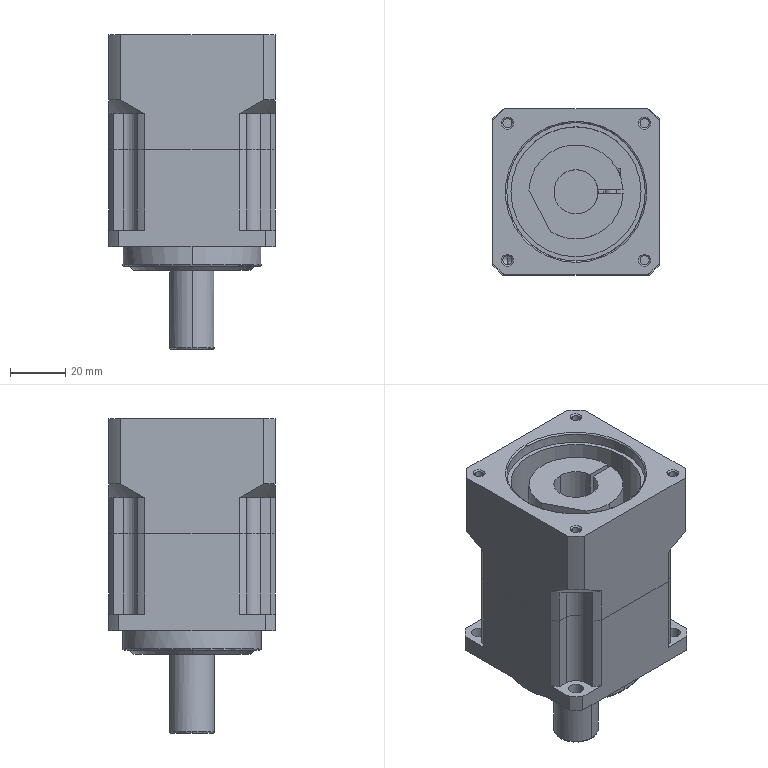Part | NX | 2 solids | 162 faces | box 60 x 60 x 113.5 mm | volume 214888 mm3 | cylinder 74 | plane 60 | cone 20 | torus 8 | commonest cylinder face diameters 69 x16 3.3 x8 5.5 x8 10 x8 16 x4 50 x4